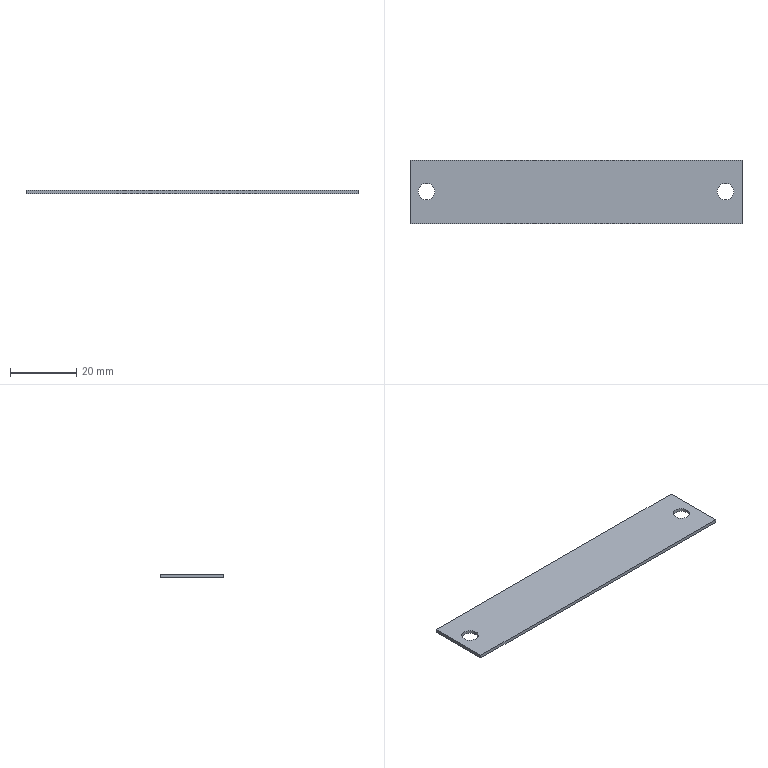Part | SolidWorks | features Extrusion 1, HoleWzd 1 | 1 solid | 10 faces | box 100 x 19 x 1 mm | volume 1861 mm3 | plane 6 | cylinder 4 | commonest cylinder face diameters 5 x4
STEP:
#1=CARTESIAN_POINT('',(-47.5,9.622,0.));
#2=VERTEX_POINT('',#1);
#3=CARTESIAN_POINT('',(-42.5,9.622,0.));
#4=VERTEX_POINT('',#3);
#5=CARTESIAN_POINT('',(-45.,9.622,0.));
#6=DIRECTION('',(0.,0.,1.));
#7=DIRECTION('',(1.,0.,0.));
#8=AXIS2_PLACEMENT_3D('',#5,#6,#7);
#9=CIRCLE('',#8,2.5);
#10=EDGE_CURVE('',#2,#4,#9,.T.);
#11=ORIENTED_EDGE('',*,*,#10,.F.);
#12=CARTESIAN_POINT('',(-47.5,9.622,1.));
#13=VERTEX_POINT('',#12);
#14=CARTESIAN_POINT('',(-47.5,9.622,1.));
#15=DIRECTION('',(0.,0.,1.));
#16=VECTOR('',#15,1000.);
#17=LINE('',#14,#16);
#18=EDGE_CURVE('',#2,#13,#17,.T.);
#19=ORIENTED_EDGE('',*,*,#18,.T.);
#20=CARTESIAN_POINT('',(-42.5,9.622,1.));
#21=VERTEX_POINT('',#20);
#22=CARTESIAN_POINT('',(-45.,9.622,1.));
#23=DIRECTION('',(0.,0.,1.));
#24=DIRECTION('',(1.,0.,0.));
#25=AXIS2_PLACEMENT_3D('',#22,#23,#24);
#26=CIRCLE('',#25,2.5);
#27=EDGE_CURVE('',#13,#21,#26,.T.);
#28=ORIENTED_EDGE('',*,*,#27,.T.);
#29=CARTESIAN_POINT('',(-42.5,9.622,1.));
#30=DIRECTION('',(0.,0.,1.));
#31=VECTOR('',#30,1000.);
#32=LINE('',#29,#31);
#33=EDGE_CURVE('',#4,#21,#32,.T.);
#34=ORIENTED_EDGE('',*,*,#33,.F.);
#35=EDGE_LOOP('',(#11,#19,#28,#34));
#36=FACE_OUTER_BOUND('',#35,.T.);
#37=CARTESIAN_POINT('',(-45.,9.622,1.));
#38=DIRECTION('',(0.,0.,1.));
#39=DIRECTION('',(1.,0.,0.));
#40=AXIS2_PLACEMENT_3D('',#37,#38,#39);
#41=CYLINDRICAL_SURFACE('',#40,2.5);
#42=ADVANCED_FACE('',(#36),#41,.F.);
#43=CARTESIAN_POINT('',(42.5,9.622,0.));
#44=VERTEX_POINT('',#43);
#45=CARTESIAN_POINT('',(47.5,9.622,0.));
#46=VERTEX_POINT('',#45);
#47=CARTESIAN_POINT('',(45.,9.622,0.));
#48=DIRECTION('',(0.,0.,1.));
#49=DIRECTION('',(1.,0.,0.));
#50=AXIS2_PLACEMENT_3D('',#47,#48,#49);
#51=CIRCLE('',#50,2.5);
#52=EDGE_CURVE('',#44,#46,#51,.T.);
#53=ORIENTED_EDGE('',*,*,#52,.F.);
#54=CARTESIAN_POINT('',(42.5,9.622,1.));
#55=VERTEX_POINT('',#54);
#56=CARTESIAN_POINT('',(42.5,9.622,1.));
#57=DIRECTION('',(0.,0.,1.));
#58=VECTOR('',#57,1000.);
#59=LINE('',#56,#58);
#60=EDGE_CURVE('',#44,#55,#59,.T.);
#61=ORIENTED_EDGE('',*,*,#60,.T.);
#62=CARTESIAN_POINT('',(47.5,9.622,1.));
#63=VERTEX_POINT('',#62);
#64=CARTESIAN_POINT('',(45.,9.622,1.));
#65=DIRECTION('',(0.,0.,1.));
#66=DIRECTION('',(1.,0.,0.));
#67=AXIS2_PLACEMENT_3D('',#64,#65,#66);
#68=CIRCLE('',#67,2.5);
#69=EDGE_CURVE('',#55,#63,#68,.T.);
#70=ORIENTED_EDGE('',*,*,#69,.T.);
#71=CARTESIAN_POINT('',(47.5,9.622,1.));
#72=DIRECTION('',(0.,0.,1.));
#73=VECTOR('',#72,1000.);
#74=LINE('',#71,#73);
#75=EDGE_CURVE('',#46,#63,#74,.T.);
#76=ORIENTED_EDGE('',*,*,#75,.F.);
#77=EDGE_LOOP('',(#53,#61,#70,#76));
#78=FACE_OUTER_BOUND('',#77,.T.);
#79=CARTESIAN_POINT('',(45.,9.622,1.));
#80=DIRECTION('',(0.,0.,1.));
#81=DIRECTION('',(1.,0.,0.));
#82=AXIS2_PLACEMENT_3D('',#79,#80,#81);
#83=CYLINDRICAL_SURFACE('',#82,2.5);
#84=ADVANCED_FACE('',(#78),#83,.F.);
#85=CARTESIAN_POINT('',(-50.,19.,0.));
#86=VERTEX_POINT('',#85);
#87=CARTESIAN_POINT('',(-50.,0.,0.));
#88=VERTEX_POINT('',#87);
#89=CARTESIAN_POINT('',(-50.,19.,0.));
#90=DIRECTION('',(0.,-1.,0.));
#91=VECTOR('',#90,1000.);
#92=LINE('',#89,#91);
#93=EDGE_CURVE('',#86,#88,#92,.T.);
#94=ORIENTED_EDGE('',*,*,#93,.T.);
#95=CARTESIAN_POINT('',(-50.,0.,1.));
#96=VERTEX_POINT('',#95);
#97=CARTESIAN_POINT('',(-50.,0.,1.));
#98=DIRECTION('',(0.,0.,-1.));
#99=VECTOR('',#98,1000.);
#100=LINE('',#97,#99);
#101=EDGE_CURVE('',#96,#88,#100,.T.);
#102=ORIENTED_EDGE('',*,*,#101,.F.);
#103=CARTESIAN_POINT('',(-50.,19.,1.));
#104=VERTEX_POINT('',#103);
#105=CARTESIAN_POINT('',(-50.,19.,1.));
#106=DIRECTION('',(0.,-1.,0.));
#107=VECTOR('',#106,1000.);
#108=LINE('',#105,#107);
#109=EDGE_CURVE('',#104,#96,#108,.T.);
#110=ORIENTED_EDGE('',*,*,#109,.F.);
#111=CARTESIAN_POINT('',(-50.,19.,1.));
#112=DIRECTION('',(0.,0.,-1.));
#113=VECTOR('',#112,1000.);
#114=LINE('',#111,#113);
#115=EDGE_CURVE('',#104,#86,#114,.T.);
#116=ORIENTED_EDGE('',*,*,#115,.T.);
#117=EDGE_LOOP('',(#94,#102,#110,#116));
#118=FACE_OUTER_BOUND('',#117,.T.);
#119=CARTESIAN_POINT('',(-50.,19.,1.));
#120=DIRECTION('',(1.,0.,0.));
#121=DIRECTION('',(0.,0.,-1.));
#122=AXIS2_PLACEMENT_3D('',#119,#120,#121);
#123=PLANE('',#122);
#124=ADVANCED_FACE('',(#118),#123,.F.);
#125=CARTESIAN_POINT('',(50.,0.,0.));
#126=VERTEX_POINT('',#125);
#127=CARTESIAN_POINT('',(-50.,0.,0.));
#128=DIRECTION('',(1.,0.,0.));
#129=VECTOR('',#128,1000.);
#130=LINE('',#127,#129);
#131=EDGE_CURVE('',#88,#126,#130,.T.);
#132=ORIENTED_EDGE('',*,*,#131,.T.);
#133=CARTESIAN_POINT('',(50.,0.,1.));
#134=VERTEX_POINT('',#133);
#135=CARTESIAN_POINT('',(50.,0.,1.));
#136=DIRECTION('',(0.,0.,-1.));
#137=VECTOR('',#136,1000.);
#138=LINE('',#135,#137);
#139=EDGE_CURVE('',#134,#126,#138,.T.);
#140=ORIENTED_EDGE('',*,*,#139,.F.);
#141=CARTESIAN_POINT('',(-50.,0.,1.));
#142=DIRECTION('',(1.,0.,0.));
#143=VECTOR('',#142,1000.);
#144=LINE('',#141,#143);
#145=EDGE_CURVE('',#96,#134,#144,.T.);
#146=ORIENTED_EDGE('',*,*,#145,.F.);
#147=ORIENTED_EDGE('',*,*,#101,.T.);
#148=EDGE_LOOP('',(#132,#140,#146,#147));
#149=FACE_OUTER_BOUND('',#148,.T.);
#150=CARTESIAN_POINT('',(-50.,0.,1.));
#151=DIRECTION('',(0.,1.,0.));
#152=DIRECTION('',(0.,0.,1.));
#153=AXIS2_PLACEMENT_3D('',#150,#151,#152);
#154=PLANE('',#153);
#155=ADVANCED_FACE('',(#149),#154,.F.);
#156=CARTESIAN_POINT('',(50.,19.,0.));
#157=VERTEX_POINT('',#156);
#158=CARTESIAN_POINT('',(50.,19.,0.));
#159=DIRECTION('',(0.,1.,0.));
#160=VECTOR('',#159,1000.);
#161=LINE('',#158,#160);
#162=EDGE_CURVE('',#126,#157,#161,.T.);
#163=ORIENTED_EDGE('',*,*,#162,.T.);
#164=CARTESIAN_POINT('',(50.,19.,1.));
#165=VERTEX_POINT('',#164);
#166=CARTESIAN_POINT('',(50.,19.,1.));
#167=DIRECTION('',(0.,0.,-1.));
#168=VECTOR('',#167,1000.);
#169=LINE('',#166,#168);
#170=EDGE_CURVE('',#165,#157,#169,.T.);
#171=ORIENTED_EDGE('',*,*,#170,.F.);
#172=CARTESIAN_POINT('',(50.,19.,1.));
#173=DIRECTION('',(0.,1.,0.));
#174=VECTOR('',#173,1000.);
#175=LINE('',#172,#174);
#176=EDGE_CURVE('',#134,#165,#175,.T.);
#177=ORIENTED_EDGE('',*,*,#176,.F.);
#178=ORIENTED_EDGE('',*,*,#139,.T.);
#179=EDGE_LOOP('',(#163,#171,#177,#178));
#180=FACE_OUTER_BOUND('',#179,.T.);
#181=CARTESIAN_POINT('',(50.,19.,1.));
#182=DIRECTION('',(-1.,0.,0.));
#183=DIRECTION('',(0.,0.,1.));
#184=AXIS2_PLACEMENT_3D('',#181,#182,#183);
#185=PLANE('',#184);
#186=ADVANCED_FACE('',(#180),#185,.F.);
#187=CARTESIAN_POINT('',(-50.,19.,0.));
#188=DIRECTION('',(-1.,0.,0.));
#189=VECTOR('',#188,1000.);
#190=LINE('',#187,#189);
#191=EDGE_CURVE('',#157,#86,#190,.T.);
#192=ORIENTED_EDGE('',*,*,#191,.T.);
#193=ORIENTED_EDGE('',*,*,#115,.F.);
#194=CARTESIAN_POINT('',(-50.,19.,1.));
#195=DIRECTION('',(-1.,0.,0.));
#196=VECTOR('',#195,1000.);
#197=LINE('',#194,#196);
#198=EDGE_CURVE('',#165,#104,#197,.T.);
#199=ORIENTED_EDGE('',*,*,#198,.F.);
#200=ORIENTED_EDGE('',*,*,#170,.T.);
#201=EDGE_LOOP('',(#192,#193,#199,#200));
#202=FACE_OUTER_BOUND('',#201,.T.);
#203=CARTESIAN_POINT('',(-50.,19.,1.));
#204=DIRECTION('',(0.,-1.,0.));
#205=DIRECTION('',(0.,0.,-1.));
#206=AXIS2_PLACEMENT_3D('',#203,#204,#205);
#207=PLANE('',#206);
#208=ADVANCED_FACE('',(#202),#207,.F.);
#209=CARTESIAN_POINT('',(-45.,9.622,1.));
#210=DIRECTION('',(0.,0.,1.));
#211=DIRECTION('',(1.,0.,0.));
#212=AXIS2_PLACEMENT_3D('',#209,#210,#211);
#213=CIRCLE('',#212,2.5);
#214=EDGE_CURVE('',#21,#13,#213,.T.);
#215=ORIENTED_EDGE('',*,*,#214,.F.);
#216=ORIENTED_EDGE('',*,*,#27,.F.);
#217=EDGE_LOOP('',(#215,#216));
#218=FACE_BOUND('',#217,.T.);
#219=CARTESIAN_POINT('',(45.,9.622,1.));
#220=DIRECTION('',(0.,0.,1.));
#221=DIRECTION('',(1.,0.,0.));
#222=AXIS2_PLACEMENT_3D('',#219,#220,#221);
#223=CIRCLE('',#222,2.5);
#224=EDGE_CURVE('',#63,#55,#223,.T.);
#225=ORIENTED_EDGE('',*,*,#224,.F.);
#226=ORIENTED_EDGE('',*,*,#69,.F.);
#227=EDGE_LOOP('',(#225,#226));
#228=FACE_BOUND('',#227,.T.);
#229=ORIENTED_EDGE('',*,*,#109,.T.);
#230=ORIENTED_EDGE('',*,*,#145,.T.);
#231=ORIENTED_EDGE('',*,*,#176,.T.);
#232=ORIENTED_EDGE('',*,*,#198,.T.);
#233=EDGE_LOOP('',(#229,#230,#231,#232));
#234=FACE_OUTER_BOUND('',#233,.T.);
#235=CARTESIAN_POINT('',(0.,0.,1.));
#236=DIRECTION('',(0.,0.,1.));
#237=DIRECTION('',(1.,0.,0.));
#238=AXIS2_PLACEMENT_3D('',#235,#236,#237);
#239=PLANE('',#238);
#240=ADVANCED_FACE('',(#218,#228,#234),#239,.T.);
#241=CARTESIAN_POINT('',(-45.,9.622,0.));
#242=DIRECTION('',(0.,0.,1.));
#243=DIRECTION('',(1.,0.,0.));
#244=AXIS2_PLACEMENT_3D('',#241,#242,#243);
#245=CIRCLE('',#244,2.5);
#246=EDGE_CURVE('',#4,#2,#245,.T.);
#247=ORIENTED_EDGE('',*,*,#246,.T.);
#248=ORIENTED_EDGE('',*,*,#10,.T.);
#249=EDGE_LOOP('',(#247,#248));
#250=FACE_BOUND('',#249,.T.);
#251=CARTESIAN_POINT('',(45.,9.622,0.));
#252=DIRECTION('',(0.,0.,1.));
#253=DIRECTION('',(1.,0.,0.));
#254=AXIS2_PLACEMENT_3D('',#251,#252,#253);
#255=CIRCLE('',#254,2.5);
#256=EDGE_CURVE('',#46,#44,#255,.T.);
#257=ORIENTED_EDGE('',*,*,#256,.T.);
#258=ORIENTED_EDGE('',*,*,#52,.T.);
#259=EDGE_LOOP('',(#257,#258));
#260=FACE_BOUND('',#259,.T.);
#261=ORIENTED_EDGE('',*,*,#93,.F.);
#262=ORIENTED_EDGE('',*,*,#191,.F.);
#263=ORIENTED_EDGE('',*,*,#162,.F.);
#264=ORIENTED_EDGE('',*,*,#131,.F.);
#265=EDGE_LOOP('',(#261,#262,#263,#264));
#266=FACE_OUTER_BOUND('',#265,.T.);
#267=CARTESIAN_POINT('',(0.,0.,0.));
#268=DIRECTION('',(0.,0.,1.));
#269=DIRECTION('',(1.,0.,0.));
#270=AXIS2_PLACEMENT_3D('',#267,#268,#269);
#271=PLANE('',#270);
#272=ADVANCED_FACE('',(#250,#260,#266),#271,.F.);
#273=ORIENTED_EDGE('',*,*,#60,.F.);
#274=ORIENTED_EDGE('',*,*,#256,.F.);
#275=ORIENTED_EDGE('',*,*,#75,.T.);
#276=ORIENTED_EDGE('',*,*,#224,.T.);
#277=EDGE_LOOP('',(#273,#274,#275,#276));
#278=FACE_OUTER_BOUND('',#277,.T.);
#279=CARTESIAN_POINT('',(45.,9.622,1.));
#280=DIRECTION('',(0.,0.,1.));
#281=DIRECTION('',(1.,0.,0.));
#282=AXIS2_PLACEMENT_3D('',#279,#280,#281);
#283=CYLINDRICAL_SURFACE('',#282,2.5);
#284=ADVANCED_FACE('',(#278),#283,.F.);
#285=ORIENTED_EDGE('',*,*,#18,.F.);
#286=ORIENTED_EDGE('',*,*,#246,.F.);
#287=ORIENTED_EDGE('',*,*,#33,.T.);
#288=ORIENTED_EDGE('',*,*,#214,.T.);
#289=EDGE_LOOP('',(#285,#286,#287,#288));
#290=FACE_OUTER_BOUND('',#289,.T.);
#291=CARTESIAN_POINT('',(-45.,9.622,1.));
#292=DIRECTION('',(0.,0.,1.));
#293=DIRECTION('',(1.,0.,0.));
#294=AXIS2_PLACEMENT_3D('',#291,#292,#293);
#295=CYLINDRICAL_SURFACE('',#294,2.5);
#296=ADVANCED_FACE('',(#290),#295,.F.);
#297=CLOSED_SHELL('',(#42,#84,#124,#155,#186,#208,#240,#272,#284,#296));
#298=MANIFOLD_SOLID_BREP('',#297);
#299=CARTESIAN_POINT('',(0.,0.,0.));
#300=DIRECTION('',(0.,0.,1.));
#301=DIRECTION('',(1.,0.,0.));
#302=AXIS2_PLACEMENT_3D('',#299,#300,#301);
#303=(LENGTH_UNIT()NAMED_UNIT(*)SI_UNIT(.MILLI.,.METRE.));
#304=UNCERTAINTY_MEASURE_WITH_UNIT(LENGTH_MEASURE(0.00001),#303,'','');
#305=(NAMED_UNIT(*)PLANE_ANGLE_UNIT()SI_UNIT($,.RADIAN.));
#306=(NAMED_UNIT(*)SI_UNIT($,.STERADIAN.)SOLID_ANGLE_UNIT());
#307=(GEOMETRIC_REPRESENTATION_CONTEXT(3)GLOBAL_UNCERTAINTY_ASSIGNED_CONTEXT((#304))GLOBAL_UNIT_ASSIGNED_CONTEXT((#303,#305,#306))REPRESENTATION_CONTEXT('',''));
#308=ADVANCED_BREP_SHAPE_REPRESENTATION('',(#298,#302),#307);